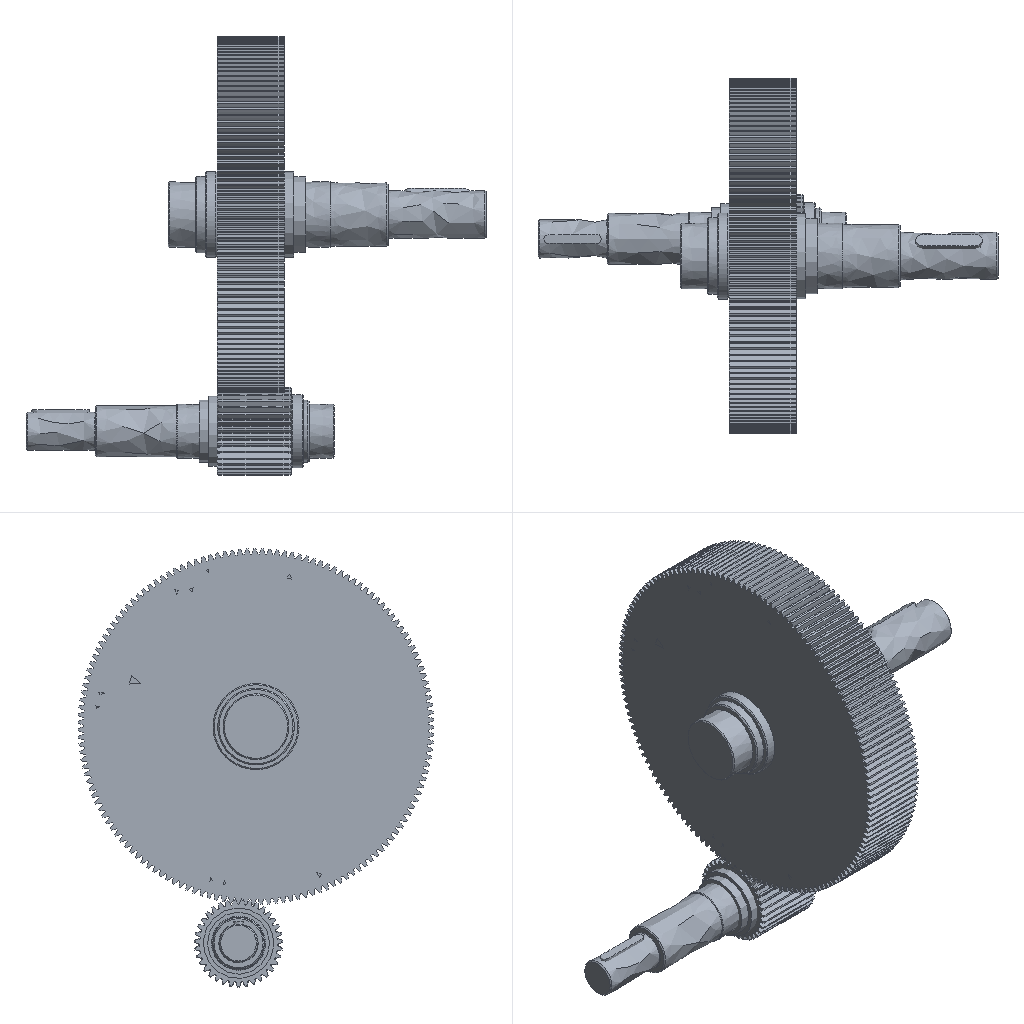Simulation study | ansys workbench
Set-up summary:
category,name,step,type,value,unit,region
solver,ansys_workbench
units,mm-N-s-tonne (MPa),,stated,"/units,MPA"
analysis,LS1,,static
load_step,LS1,LS1,static,nsubst=1; time=1
mesh,nodes,,,107579
mesh,elements,,,52101
element_type,SOLID187,,,31561
element_type,SOLID186,,,8942
element_type,CONTA174,,,5958
element_type,TARGE170,,,5640
material,Structural Steel,,E,200000,tonne s^-2 mm^-1
material,Structural Steel,,nu,0.3
material,Structural Steel,,density,7.85e-09,tonne mm^-3
material,Structural Steel,,conductivity,60.5,tonne mm s^-3 C^-1
material,Structural Steel,,specific_heat,4.34e+08,mm^2 s^-2 C^-1
material,Structural Steel,,cte,1.2e-05,C^-1
material,Structural Steel,,permeability,10000
material,Structural Steel,,resistivity,0.00017,ohm mm
load,,LS1,moment,"500 [dir=(1, 0, 0) n=3]",,all
bc,Fixed Supports,model,fixed,[dofs=ALL],,_FIXEDSU
contact,Contact Region,,bonded (always),element=CONTA174
contact,Contact Region 2,,bonded (always),element=CONTA174
contact,Contact Region 3,,bonded (always),element=CONTA174
contact,Contact Region 4,,bonded (always),element=CONTA174
contact,Contact Region 5,,bonded (always),element=CONTA174
contact,Contact Region 6,,bonded (always),element=CONTA174
contact,Contact Region 7,,bonded (always),element=CONTA174
contact,Contact Region 8,,bonded (always),element=CONTA174
contact,Contact Region 9,,bonded (always),element=CONTA174
contact,Contact Region 10,,bonded (always),element=CONTA174
contact,Contact Region 11,,bonded (always),element=CONTA174
contact,Contact Region 12,,bonded (always),element=CONTA174
contact,Contact Region 13,,bonded (always),element=CONTA174
contact,contact 14,,bonded (always),element=CONTA174
named_set,_FIXEDSU,,node,704
Ansys APDL input file, long lists of numbers shortened:
/batch
/config,noeldb,1     ! force off writing results to database
*get,_wallstrt,active,,time,wall
! ANSYS input file written by Workbench version 2022 R1
! File used for geometry attach:
/title,wbnew--____ (A5)
! ****** Begin Custom Load Command Snippet ******
/COM, ACT Extensions:
/COM,     LSDYNA, 2021.1
/COM,
! ****** End   Custom Load Command Snippet ******
*DIM,_wb_ProjectScratch_dir,string,248
_wb_ProjectScratch_dir(1) = ''
*DIM,_wb_SolverFiles_dir,string,248
_wb_SolverFiles_dir(1) = ''
*DIM,_wb_userfiles_dir,string,248
_wb_userfiles_dir(1) = ''
/com,--- Data in consistent NMM units. See Solving Units in the help system for more information.
/units,MPA
/nopr
/wb,file,start              !  signify a WB generated input file
/prep7
! Turn off shape checking because checks already performed inside WB mesher.
! See help system for more information.
SHPP,OFF,,NOWARN
/nolist
etcon,set             ! allow ANSYS to choose best KEYOP's for 180x elements, resets any applicable keyopt to MAPDL defaults
/com,*********** Nodes for the whole assembly ***********
nblock,3,,118335
(1i9,3e20.9e3)
        1     1.706495079E+02     1.993704432E+00     2.810000000E+01
! (107577 more lines like these left out)
-1
/com,*********** Nodes for all Remote Points ***********
nblock,3
(1i9,3e20.9e3)
   107579     1.897250275E+02    -5.267150244E+00     3.130672649E+01
-1
/wb,elem,start            !  set before creation of elements
/com,*********** Elements for Body 1 "_2___|_ II|__1" ***********
et,1,187
eblock,19,solid,,8572
(19i9)
        1        1        1        1        0        0        0        0       10        0    13585    28511    28512    28794    28787    41030    41045    41038    41036
! (17143 more lines like these left out)
-1
/com,*********** Elements for Body 2 "_2___|GB_T 1096-2003[____ A__ 16_10_46__ 16_10_50|__1" ***********
et,2,186
keyo,2,2,1          ! set full integration on SOLID186
eblock,19,solid,,192
(19i9)
        2        2        2        2        0        0        0        0       20        0      375     1540     1542     1550     1541     1667     1665     1657     1666
! (383 more lines like these left out)
-1
/com,*********** Elements for Body 3 "_2___|__2|__-__1" ***********
et,3,186
keyo,3,2,1          ! set full integration on SOLID186
eblock,19,solid,,8574
(19i9)
        3        3        3        3        0        0        0        0       20        0    22157    41530    44740    44442    42326    48813    47208    47357    48415
! (17147 more lines like these left out)
-1
/com,*********** Elements for Body 4 "_2___|__~_II|__1" ***********
et,4,187
eblock,19,solid,,198
(19i9)
        4        4        4        4        0        0        0        0       10        0      567     2682     2718     2710     2717     3000     3087     2998     2999
! (395 more lines like these left out)
-1
/com,*********** Elements for Body 5 "_2___|GB_T 1096-2003[____ A__ 12_8_70]__ 12_8_70|__1" ***********
et,5,187
eblock,19,solid,,3194
(19i9)
        5        5        5        5        0        0        0        0       10        0      765     3681     3968     4068     4026     7142     8824     7145     7143
! (6387 more lines like these left out)
-1
/com,*********** Elements for Body 6 "_ I|__2" ***********
et,6,187
eblock,19,solid,,7493
(19i9)
        6        6        6        6        0        0        0        0       10        0     6092    14325    15036    15226    15212    21969    26122    21972    21971
! (14985 more lines like these left out)
-1
/com,*********** Elements for Body 7 "___|__-__2" ***********
et,7,187
eblock,19,solid,,9773
(19i9)
        7        7        7        7        0        0        0        0       10        0    30731    90303    90305    92112    91357   100339   100352   100344   100341
! (19545 more lines like these left out)
-1
/com,*********** Elements for Body 8 "GB_T 1096-2003[____ A__ 10_8_50__ 10_8_50|__1" ***********
et,8,187
eblock,19,solid,,2133
(19i9)
        8        8        8        8        0        0        0        0       10        0     3959     9082     9711     9573     9694    10021    12604    10019    10020
! (4265 more lines like these left out)
-1
/com,*********** Elements for Body 9 "GB_T 1096-2003[____ A__ 14_9_56__ 14_9_56|__1" ***********
et,9,186
keyo,9,2,1          ! set full integration on SOLID186
eblock,19,solid,,176
(19i9)
        9        9        9        9        0        0        0        0       20        0        1        1        2        3       12      104      103      102       93
! (351 more lines like these left out)
-1
/com,*********** Elements for Body 10 "__~_I|__1" ***********
et,10,187
eblock,19,solid,,198
(19i9)
       10       10       10       10        0        0        0        0       10        0      177     1062     1082     1081     1071     1246     1324     1245     1243
! (395 more lines like these left out)
-1
/wb,elem,end               !  done creating elements
/com,*********** Send User Defined Coordinate System(s) ***********
csys,0
toffst,273.15,  ! Temperature offset from absolute zero
/com,*********** Set Reference Temperature ***********
tref,22.
/wb,mat,start              !  starting to send materials
/com,*********** Send Materials ***********
Temperature = 'TEMP' ! Temperature
MP,DENS,1,7.85e-09,	! tonne mm^-3
MP,ALPX,1,1.2e-05,	! C^-1
MP,C,1,434000000,	! mm^2 s^-2 C^-1
MP,KXX,1,60.5,	! tonne mm s^-3 C^-1
MP,RSVX,1,0.00017,	! ohm mm
MP,EX,1,200000,	! tonne s^-2 mm^-1
MP,NUXY,1,0.3,
MP,MURX,1,10000,
Temperature = 'TEMP' ! Temperature
MP,DENS,2,7.85e-09,	! tonne mm^-3
MP,ALPX,2,1.2e-05,	! C^-1
MP,C,2,434000000,	! mm^2 s^-2 C^-1
MP,KXX,2,60.5,	! tonne mm s^-3 C^-1
MP,RSVX,2,0.00017,	! ohm mm
MP,EX,2,200000,	! tonne s^-2 mm^-1
MP,NUXY,2,0.3,
MP,MURX,2,10000,
Temperature = 'TEMP' ! Temperature
MP,DENS,3,7.85e-09,	! tonne mm^-3
MP,ALPX,3,1.2e-05,	! C^-1
MP,C,3,434000000,	! mm^2 s^-2 C^-1
MP,KXX,3,60.5,	! tonne mm s^-3 C^-1
MP,RSVX,3,0.00017,	! ohm mm
MP,EX,3,200000,	! tonne s^-2 mm^-1
MP,NUXY,3,0.3,
MP,MURX,3,10000,
Temperature = 'TEMP' ! Temperature
MP,DENS,4,7.85e-09,	! tonne mm^-3
MP,ALPX,4,1.2e-05,	! C^-1
MP,C,4,434000000,	! mm^2 s^-2 C^-1
MP,KXX,4,60.5,	! tonne mm s^-3 C^-1
MP,RSVX,4,0.00017,	! ohm mm
MP,EX,4,200000,	! tonne s^-2 mm^-1
MP,NUXY,4,0.3,
MP,MURX,4,10000,
Temperature = 'TEMP' ! Temperature
MP,DENS,5,7.85e-09,	! tonne mm^-3
MP,ALPX,5,1.2e-05,	! C^-1
MP,C,5,434000000,	! mm^2 s^-2 C^-1
MP,KXX,5,60.5,	! tonne mm s^-3 C^-1
MP,RSVX,5,0.00017,	! ohm mm
MP,EX,5,200000,	! tonne s^-2 mm^-1
MP,NUXY,5,0.3,
MP,MURX,5,10000,
Temperature = 'TEMP' ! Temperature
MP,DENS,6,7.85e-09,	! tonne mm^-3
MP,ALPX,6,1.2e-05,	! C^-1
MP,C,6,434000000,	! mm^2 s^-2 C^-1
MP,KXX,6,60.5,	! tonne mm s^-3 C^-1
MP,RSVX,6,0.00017,	! ohm mm
MP,EX,6,200000,	! tonne s^-2 mm^-1
MP,NUXY,6,0.3,
MP,MURX,6,10000,
Temperature = 'TEMP' ! Temperature
MP,DENS,7,7.85e-09,	! tonne mm^-3
MP,ALPX,7,1.2e-05,	! C^-1
MP,C,7,434000000,	! mm^2 s^-2 C^-1
MP,KXX,7,60.5,	! tonne mm s^-3 C^-1
MP,RSVX,7,0.00017,	! ohm mm
MP,EX,7,200000,	! tonne s^-2 mm^-1
MP,NUXY,7,0.3,
MP,MURX,7,10000,
Temperature = 'TEMP' ! Temperature
MP,DENS,8,7.85e-09,	! tonne mm^-3
MP,ALPX,8,1.2e-05,	! C^-1
MP,C,8,434000000,	! mm^2 s^-2 C^-1
MP,KXX,8,60.5,	! tonne mm s^-3 C^-1
MP,RSVX,8,0.00017,	! ohm mm
MP,EX,8,200000,	! tonne s^-2 mm^-1
MP,NUXY,8,0.3,
MP,MURX,8,10000,
Temperature = 'TEMP' ! Temperature
MP,DENS,9,7.85e-09,	! tonne mm^-3
MP,ALPX,9,1.2e-05,	! C^-1
MP,C,9,434000000,	! mm^2 s^-2 C^-1
MP,KXX,9,60.5,	! tonne mm s^-3 C^-1
MP,RSVX,9,0.00017,	! ohm mm
MP,EX,9,200000,	! tonne s^-2 mm^-1
MP,NUXY,9,0.3,
MP,MURX,9,10000,
Temperature = 'TEMP' ! Temperature
MP,DENS,10,7.85e-09,	! tonne mm^-3
MP,ALPX,10,1.2e-05,	! C^-1
MP,C,10,434000000,	! mm^2 s^-2 C^-1
MP,KXX,10,60.5,	! tonne mm s^-3 C^-1
MP,RSVX,10,0.00017,	! ohm mm
MP,EX,10,200000,	! tonne s^-2 mm^-1
MP,NUXY,10,0.3,
MP,MURX,10,10000,
/wb,mat,end                !  done sending materials
!************************* Model Summary ********************
!_2___|_ II|__1,	结构钢,	matid,	1
!_2___|GB_T 1096-2003[____ A__ 16_10_46__ 16_10_50|__1,	结构钢,	matid,	2
!_2___|__2|__-__1,	结构钢,	matid,	3
!_2___|__~_II|__1,	结构钢,	matid,	4
!_2___|GB_T 1096-2003[____ A__ 12_8_70]__ 12_8_70|__1,	结构钢,	matid,	5
!_ I|__2,	结构钢,	matid,	6
!___|__-__2,	结构钢,	matid,	7
!GB_T 1096-2003[____ A__ 10_8_50__ 10_8_50|__1,	结构钢,	matid,	8
!GB_T 1096-2003[____ A__ 14_9_56__ 14_9_56|__1,	结构钢,	matid,	9
!__~_I|__1,	结构钢,	matid,	10
!************************* End Model Summary ********************
! get the diagonal of the bounding box. Needed later for other things
*get,_xmin,node,,mnloc,x
*get,_ymin,node,,mnloc,y
*get,_zmin,node,,mnloc,z
*get,_xmax,node,,mxloc,x
*get,_ymax,node,,mxloc,y
*get,_zmax,node,,mxloc,z
_ASMDIAG=(_xmax-_xmin)*(_xmax-_xmin)+(_ymax-_ymin)*(_ymax-_ymin)+(_zmax-_zmin)*(_zmax-_zmin)
_ASMDIAG=SQRT(_ASMDIAG)
/wb,contact,start          !  starting to send contact
/com,*********** Create Contact "接触区域" ***********
/com,            Real Constant Set For Above Contact Is 12 & 11
*set,tid,12
*set,cid,11
r,tid
r,cid
et,tid,170
et,cid,174
eblock,10,,,46
(15i9)
    63849       12       12       12        0    26772    26768    26773    26773    31125    31126    26773    31154
! (45 more lines like these left out)
-1
eblock,10,,,46
(15i9)
    63895       11       11       11        0    26772    26768    26773    26773    31125    31126    26773    31154
! (45 more lines like these left out)
-1
eblock,10,,,150
(15i9)
    63941       11       12       11        0     1727     1711     1720     1719     2385     2383     2407     2408
! (149 more lines like these left out)
-1
eblock,10,,,150
(15i9)
    64091       12       11       12        0     1727     1711     1720     1719     2385     2383     2407     2408
! (149 more lines like these left out)
-1
keyo,cid,8,2               ! auto create asymmetric contact (from Program Controlled setting)
keyo,cid,10,0              ! adjust contact stiffness each NR iteration (from Program Controlled setting)
keyo,cid,12,5              ! bonded always
keyo,cid,18,1              ! small sliding turned on by application
keyo,cid,2,0               ! augmented Lagrange (from Program Controlled setting)
keyo,cid,4,0               ! on Gauss point (from Program Controlled setting)
keyo,cid,9,1               ! ignore initial gaps/penetration
keyo,cid,7,0               ! No Prediction
rmod,tid,3,10.      ! FKN
rmod,tid,5,0.       ! ICONT
rmod,tid,6,0.       ! PINB
rmod,tid,10,0.      ! CNOF
rmod,tid,12,0.      ! FKT
rmod,tid,36,53      ! WB DSID
rmod,cid,3,10.      ! FKN
rmod,cid,5,0.       ! ICONT
rmod,cid,6,0.       ! PINB
rmod,cid,10,0.      ! CNOF
rmod,cid,12,0.      ! FKT
rmod,cid,36,53      ! WB DSID
/com,*********** Create Contact "接触区域 2" ***********
/com,            Real Constant Set For Above Contact Is 14 & 13
*set,tid,14
*set,cid,13
r,tid
r,cid
et,tid,170
et,cid,174
eblock,10,,,557
(15i9)
    64241       14       14       14        0    26368    26375    27732    27732    28892    28986    27732    28899
! (556 more lines like these left out)
-1
eblock,10,,,557
(15i9)
    64798       13       13       13        0    26368    26375    27732    27732    28892    28986    27732    28899
! (556 more lines like these left out)
-1
eblock,10,,,56
(15i9)
    65355       13       14       13        0    52103    52092    52098    52099    84320    84319    84331    84333
! (55 more lines like these left out)
-1
eblock,10,,,56
(15i9)
    65411       14       13       14        0    52103    52092    52098    52099    84320    84319    84331    84333
! (55 more lines like these left out)
-1
keyo,cid,8,2               ! auto create asymmetric contact (from Program Controlled setting)
keyo,cid,10,0              ! adjust contact stiffness each NR iteration (from Program Controlled setting)
keyo,cid,12,5              ! bonded always
keyo,cid,18,1              ! small sliding turned on by application
keyo,cid,2,0               ! augmented Lagrange (from Program Controlled setting)
keyo,cid,4,0               ! on Gauss point (from Program Controlled setting)
keyo,cid,9,1               ! ignore initial gaps/penetration
keyo,cid,7,0               ! No Prediction
rmod,tid,3,10.      ! FKN
rmod,tid,5,0.       ! ICONT
rmod,tid,6,0.       ! PINB
rmod,tid,10,0.      ! CNOF
rmod,tid,12,0.      ! FKT
rmod,tid,36,56      ! WB DSID
rmod,cid,3,10.      ! FKN
rmod,cid,5,0.       ! ICONT
rmod,cid,6,0.       ! PINB
rmod,cid,10,0.      ! CNOF
rmod,cid,12,0.      ! FKT
rmod,cid,36,56      ! WB DSID
/com,*********** Create Contact "接触区域 3" ***********
/com,            Real Constant Set For Above Contact Is 16 & 15
*set,tid,16
*set,cid,15
r,tid
r,cid
et,tid,170
et,cid,174
eblock,10,,,144
(15i9)
    65467       16       16       16        0    27296    27687    28003    28003    34416    36123    28003    34417
! (143 more lines like these left out)
-1
eblock,10,,,144
(15i9)
    65611       15       15       15        0    27296    27687    28003    28003    34416    36123    28003    34417
! (143 more lines like these left out)
-1
eblock,10,,,32
(15i9)
    65755       15       16       15        0     2669     2678     2671     2671     2921     2929     2671     2920
! (31 more lines like these left out)
-1
eblock,10,,,32
(15i9)
    65787       16       15       16        0     2669     2678     2671     2671     2921     2929     2671     2920
! (31 more lines like these left out)
-1
keyo,cid,8,2               ! auto create asymmetric contact (from Program Controlled setting)
keyo,cid,10,0              ! adjust contact stiffness each NR iteration (from Program Controlled setting)
keyo,cid,12,5              ! bonded always
keyo,cid,18,1              ! small sliding turned on by application
keyo,cid,2,0               ! augmented Lagrange (from Program Controlled setting)
keyo,cid,4,0               ! on Gauss point (from Program Controlled setting)
keyo,cid,9,1               ! ignore initial gaps/penetration
keyo,cid,7,0               ! No Prediction
rmod,tid,3,10.      ! FKN
rmod,tid,5,0.       ! ICONT
rmod,tid,6,0.       ! PINB
rmod,tid,10,0.      ! CNOF
rmod,tid,12,0.      ! FKT
rmod,tid,36,59      ! WB DSID
rmod,cid,3,10.      ! FKN
rmod,cid,5,0.       ! ICONT
rmod,cid,6,0.       ! PINB
rmod,cid,10,0.      ! CNOF
rmod,cid,12,0.      ! FKT
rmod,cid,36,59      ! WB DSID
/com,*********** Create Contact "接触区域 4" ***********
/com,            Real Constant Set For Above Contact Is 18 & 17
*set,tid,18
*set,cid,17
r,tid
r,cid
et,tid,170
et,cid,174
eblock,10,,,44
(15i9)
    65819       18       18       18        0    26778    26774    26779    26779    31174    31175    26779    31195
! (43 more lines like these left out)
-1
eblock,10,,,44
(15i9)
    65863       17       17       17        0    26778    26774    26779    26779    31174    31175    26779    31195
! (43 more lines like these left out)
-1
eblock,10,,,954
(15i9)
    65907       17       18       17        0     3139     3374     3382     3382     4208     5781     3382     4209
! (953 more lines like these left out)
-1
eblock,10,,,954
(15i9)
    66861       18       17       18        0     3139     3374     3382     3382     4208     5781     3382     4209
! (953 more lines like these left out)
-1
keyo,cid,8,2               ! auto create asymmetric contact (from Program Controlled setting)
keyo,cid,10,0              ! adjust contact stiffness each NR iteration (from Program Controlled setting)
keyo,cid,12,5              ! bonded always
keyo,cid,18,1              ! small sliding turned on by application
keyo,cid,2,0               ! augmented Lagrange (from Program Controlled setting)
keyo,cid,4,0               ! on Gauss point (from Program Controlled setting)
keyo,cid,9,1               ! ignore initial gaps/penetration
keyo,cid,7,0               ! No Prediction
rmod,tid,3,10.      ! FKN
rmod,tid,5,0.       ! ICONT
rmod,tid,6,0.       ! PINB
rmod,tid,10,0.      ! CNOF
rmod,tid,12,0.      ! FKT
rmod,tid,36,62      ! WB DSID
rmod,cid,3,10.      ! FKN
rmod,cid,5,0.       ! ICONT
rmod,cid,6,0.       ! PINB
rmod,cid,10,0.      ! CNOF
rmod,cid,12,0.      ! FKT
rmod,cid,36,62      ! WB DSID
/com,*********** Create Contact "接触区域 5" ***********
/com,            Real Constant Set For Above Contact Is 20 & 19
*set,tid,20
*set,cid,19
r,tid
r,cid
et,tid,170
et,cid,174
eblock,10,,,150
(15i9)
    67815       20       20       20        0     1699     1700     1709     1710     2356     2359     2378     2357
! (149 more lines like these left out)
-1
eblock,10,,,150
(15i9)
    67965       19       19       19        0     1699     1700     1709     1710     2356     2359     2378     2357
! (149 more lines like these left out)
-1
eblock,10,,,12
(15i9)
    68115       19       20       19        0    54641    54640    54638    54635    89019    89017    89013    89014
! (11 more lines like these left out)
-1
eblock,10,,,12
(15i9)
    68127       20       19       20        0    54641    54640    54638    54635    89019    89017    89013    89014
! (11 more lines like these left out)
-1
keyo,cid,8,2               ! auto create asymmetric contact (from Program Controlled setting)
keyo,cid,10,0              ! adjust contact stiffness each NR iteration (from Program Controlled setting)
keyo,cid,12,5              ! bonded always
keyo,cid,18,1              ! small sliding turned on by application
keyo,cid,2,0               ! augmented Lagrange (from Program Controlled setting)
keyo,cid,4,0               ! on Gauss point (from Program Controlled setting)
keyo,cid,9,1               ! ignore initial gaps/penetration
keyo,cid,7,0               ! No Prediction
rmod,tid,3,10.      ! FKN
rmod,tid,5,0.       ! ICONT
rmod,tid,6,0.       ! PINB
rmod,tid,10,0.      ! CNOF
rmod,tid,12,0.      ! FKT
rmod,tid,36,65      ! WB DSID
rmod,cid,3,10.      ! FKN
rmod,cid,5,0.       ! ICONT
rmod,cid,6,0.       ! PINB
rmod,cid,10,0.      ! CNOF
rmod,cid,12,0.      ! FKT
rmod,cid,36,65      ! WB DSID
/com,*********** Create Contact "接触区域 6" ***********
/com,            Real Constant Set For Above Contact Is 22 & 21
*set,tid,22
*set,cid,21
r,tid
r,cid
et,tid,170
et,cid,174
eblock,10,,,27
(15i9)
    68139       22       22       22        0    48243    48759    48254    48789    76861    76882    76883    76862
! (26 more lines like these left out)
-1
eblock,10,,,27
(15i9)
    68166       21       21       21        0    48243    48759    48254    48789    76861    76882    76883    76862
! (26 more lines like these left out)
-1
eblock,10,,,32
(15i9)
    68193       21       22       21        0     2682     2701     2702     2702     2996     3052     2702     2997
! (31 more lines like these left out)
-1
eblock,10,,,32
(15i9)
    68225       22       21       22        0     2682     2701     2702     2702     2996     3052     2702     2997
! (31 more lines like these left out)
-1
keyo,cid,8,2               ! auto create asymmetric contact (from Program Controlled setting)
keyo,cid,10,0              ! adjust contact stiffness each NR iteration (from Program Controlled setting)
keyo,cid,12,5              ! bonded always
keyo,cid,18,1              ! small sliding turned on by application
keyo,cid,2,0               ! augmented Lagrange (from Program Controlled setting)
keyo,cid,4,0               ! on Gauss point (from Program Controlled setting)
keyo,cid,9,1               ! ignore initial gaps/penetration
keyo,cid,7,0               ! No Prediction
rmod,tid,3,10.      ! FKN
rmod,tid,5,0.       ! ICONT
rmod,tid,6,0.       ! PINB
rmod,tid,10,0.      ! CNOF
rmod,tid,12,0.      ! FKT
rmod,tid,36,68      ! WB DSID
rmod,cid,3,10.      ! FKN
rmod,cid,5,0.       ! ICONT
rmod,cid,6,0.       ! PINB
rmod,cid,10,0.      ! CNOF
rmod,cid,12,0.      ! FKT
rmod,cid,36,68      ! WB DSID
/com,*********** Create Contact "接触区域 7" ***********
/com,            Real Constant Set For Above Contact Is 24 & 23
*set,tid,24
*set,cid,23
r,tid
r,cid
et,tid,170
et,cid,174
eblock,10,,,51
(15i9)
    68257       24       24       24        0    52658    52661    52657    52656    85632    85629    85626    85627
! (50 more lines like these left out)
-1
eblock,10,,,51
(15i9)
    68308       23       23       23        0    52658    52661    52657    52656    85632    85629    85626    85627
! (50 more lines like these left out)
-1
eblock,10,,,300
(15i9)
    68359       23       24       23        0    89360    90371    90359    90359    94249   100564    90359    94248
! (299 more lines like these left out)
-1
eblock,10,,,300
(15i9)
    68659       24       23       24        0    89360    90371    90359    90359    94249   100564    90359    94248
! (299 more lines like these left out)
-1
keyo,cid,8,2               ! auto create asymmetric contact (from Program Controlled setting)
keyo,cid,10,0              ! adjust contact stiffness each NR iteration (from Program Controlled setting)
keyo,cid,12,5              ! bonded always
keyo,cid,18,1              ! small sliding turned on by application
keyo,cid,2,0               ! augmented Lagrange (from Program Controlled setting)
keyo,cid,4,0               ! on Gauss point (from Program Controlled setting)
keyo,cid,9,1               ! ignore initial gaps/penetration
keyo,cid,7,0               ! No Prediction
rmod,tid,3,10.      ! FKN
rmod,tid,5,0.       ! ICONT
rmod,tid,6,0.       ! PINB
rmod,tid,10,0.      ! CNOF
rmod,tid,12,0.      ! FKT
rmod,tid,36,71      ! WB DSID
rmod,cid,3,10.      ! FKN
rmod,cid,5,0.       ! ICONT
rmod,cid,6,0.       ! PINB
rmod,cid,10,0.      ! CNOF
rmod,cid,12,0.      ! FKT
rmod,cid,36,71      ! WB DSID
/com,*********** Create Contact "接触区域 8" ***********
/com,            Real Constant Set For Above Contact Is 26 & 25
*set,tid,26
*set,cid,25
r,tid
r,cid
et,tid,170
et,cid,174
eblock,10,,,572
(15i9)
    68959       26       26       26        0    14300    14296    14016    14016    21826    20532    14016    20533
! (571 more lines like these left out)
-1
eblock,10,,,572
(15i9)
    69531       25       25       25        0    14300    14296    14016    14016    21826    20532    14016    20533
! (571 more lines like these left out)
-1
eblock,10,,,617
(15i9)
    70103       25       26       25        0    89327    89328    90325    90325    94035    94043    90325    94039
! (616 more lines like these left out)
-1
eblock,10,,,617
(15i9)
    70720       26       25       26        0    89327    89328    90325    90325    94035    94043    90325    94039
! (616 more lines like these left out)
-1
keyo,cid,8,2               ! auto create asymmetric contact (from Program Controlled setting)
keyo,cid,10,0              ! adjust contact stiffness each NR iteration (from Program Controlled setting)
keyo,cid,12,5              ! bonded always
keyo,cid,18,1              ! small sliding turned on by application
keyo,cid,2,0               ! augmented Lagrange (from Program Controlled setting)
keyo,cid,4,0               ! on Gauss point (from Program Controlled setting)
keyo,cid,9,1               ! ignore initial gaps/penetration
keyo,cid,7,0               ! No Prediction
rmod,tid,3,10.      ! FKN
rmod,tid,5,0.       ! ICONT
rmod,tid,6,0.       ! PINB
rmod,tid,10,0.      ! CNOF
rmod,tid,12,0.      ! FKT
rmod,tid,36,74      ! WB DSID
rmod,cid,3,10.      ! FKN
rmod,cid,5,0.       ! ICONT
rmod,cid,6,0.       ! PINB
rmod,cid,10,0.      ! CNOF
rmod,cid,12,0.      ! FKT
rmod,cid,36,74      ! WB DSID
/com,*********** Create Contact "接触区域 9" ***********
/com,            Real Constant Set For Above Contact Is 28 & 27
*set,tid,28
*set,cid,27
r,tid
r,cid
et,tid,170
et,cid,174
eblock,10,,,44
(15i9)
    71337       28       28       28        0    13453    13452    13448    13448    17227    17203    13448    17204
! (43 more lines like these left out)
-1
eblock,10,,,44
(15i9)
    71381       27       27       27        0    13453    13452    13448    13448    17227    17203    13448    17204
! (43 more lines like these left out)
-1
eblock,10,,,690
(15i9)
    71425       27       28       27        0     9275     9063     9167     9167     9888     9887     9167    10549
! (689 more lines like these left out)
-1
eblock,10,,,690
(15i9)
    72115       28       27       28        0     9275     9063     9167     9167     9888     9887     9167    10549
! (689 more lines like these left out)
-1
keyo,cid,8,2               ! auto create asymmetric contact (from Program Controlled setting)
keyo,cid,10,0              ! adjust contact stiffness each NR iteration (from Program Controlled setting)
keyo,cid,12,5              ! bonded always
keyo,cid,18,1              ! small sliding turned on by application
keyo,cid,2,0               ! augmented Lagrange (from Program Controlled setting)
keyo,cid,4,0               ! on Gauss point (from Program Controlled setting)
keyo,cid,9,1               ! ignore initial gaps/penetration
keyo,cid,7,0               ! No Prediction
rmod,tid,3,10.      ! FKN
rmod,tid,5,0.       ! ICONT
rmod,tid,6,0.       ! PINB
rmod,tid,10,0.      ! CNOF
rmod,tid,12,0.      ! FKT
rmod,tid,36,77      ! WB DSID
rmod,cid,3,10.      ! FKN
rmod,cid,5,0.       ! ICONT
rmod,cid,6,0.       ! PINB
rmod,cid,10,0.      ! CNOF
rmod,cid,12,0.      ! FKT
rmod,cid,36,77      ! WB DSID
/com,*********** Create Contact "接触区域 10" ***********
/com,            Real Constant Set For Above Contact Is 30 & 29
*set,tid,30
*set,cid,29
r,tid
r,cid
et,tid,170
et,cid,174
eblock,10,,,44
(15i9)
    72805       30       30       30        0    13216    13212    13217    13217    15999    16000    13217    16033
! (43 more lines like these left out)
-1
eblock,10,,,44
(15i9)
    72849       29       29       29        0    13216    13212    13217    13217    15999    16000    13217    16033
! (43 more lines like these left out)
-1
eblock,10,,,154
(15i9)
    72893       29       30       29        0      181      168      176      175      820      819      832      833
! (153 more lines like these left out)
-1
eblock,10,,,154
(15i9)
    73047       30       29       30        0      181      168      176      175      820      819      832      833
! (153 more lines like these left out)
-1
keyo,cid,8,2               ! auto create asymmetric contact (from Program Controlled setting)
keyo,cid,10,0              ! adjust contact stiffness each NR iteration (from Program Controlled setting)
keyo,cid,12,5              ! bonded always
keyo,cid,18,1              ! small sliding turned on by application
keyo,cid,2,0               ! augmented Lagrange (from Program Controlled setting)
keyo,cid,4,0               ! on Gauss point (from Program Controlled setting)
keyo,cid,9,1               ! ignore initial gaps/penetration
keyo,cid,7,0               ! No Prediction
rmod,tid,3,10.      ! FKN
rmod,tid,5,0.       ! ICONT
rmod,tid,6,0.       ! PINB
rmod,tid,10,0.      ! CNOF
rmod,tid,12,0.      ! FKT
rmod,tid,36,80      ! WB DSID
rmod,cid,3,10.      ! FKN
rmod,cid,5,0.       ! ICONT
rmod,cid,6,0.       ! PINB
rmod,cid,10,0.      ! CNOF
rmod,cid,12,0.      ! FKT
rmod,cid,36,80      ! WB DSID
/com,*********** Create Contact "接触区域 11" ***********
/com,            Real Constant Set For Above Contact Is 32 & 31
*set,tid,32
*set,cid,31
r,tid
r,cid
et,tid,170
et,cid,174
eblock,10,,,138
(15i9)
    73201       32       32       32        0    13469    14223    14547    14547    17390    21466    14547    17391
! (137 more lines like these left out)
-1
eblock,10,,,138
(15i9)
    73339       31       31       31        0    13469    14223    14547    14547    17390    21466    14547    17391
! (137 more lines like these left out)
-1
eblock,10,,,32
(15i9)
    73477       31       32       31        0     1086     1095     1088     1088     1338     1346     1088     1337
! (31 more lines like these left out)
-1
eblock,10,,,32
(15i9)
    73509       32       31       32        0     1086     1095     1088     1088     1338     1346     1088     1337
! (31 more lines like these left out)
-1
keyo,cid,8,2               ! auto create asymmetric contact (from Program Controlled setting)
keyo,cid,10,0              ! adjust contact stiffness each NR iteration (from Program Controlled setting)
keyo,cid,12,5              ! bonded always
keyo,cid,18,1              ! small sliding turned on by application
keyo,cid,2,0               ! augmented Lagrange (from Program Controlled setting)
keyo,cid,4,0               ! on Gauss point (from Program Controlled setting)
keyo,cid,9,1               ! ignore initial gaps/penetration
keyo,cid,7,0               ! No Prediction
rmod,tid,3,10.      ! FKN
rmod,tid,5,0.       ! ICONT
rmod,tid,6,0.       ! PINB
rmod,tid,10,0.      ! CNOF
rmod,tid,12,0.      ! FKT
rmod,tid,36,83      ! WB DSID
rmod,cid,3,10.      ! FKN
rmod,cid,5,0.       ! ICONT
rmod,cid,6,0.       ! PINB
rmod,cid,10,0.      ! CNOF
rmod,cid,12,0.      ! FKT
rmod,cid,36,83      ! WB DSID
/com,*********** Create Contact "接触区域 12" ***********
/com,            Real Constant Set For Above Contact Is 34 & 33
*set,tid,34
*set,cid,33
r,tid
r,cid
et,tid,170
et,cid,174
eblock,10,,,52
(15i9)
    73541       34       34       34        0    89044    91311    90036    90036    92413    99210    90036    92411
! (51 more lines like these left out)
-1
eblock,10,,,52
(15i9)
    73593       33       33       33        0    89044    91311    90036    90036    92413    99210    90036    92411
! (51 more lines like these left out)
-1
eblock,10,,,162
(15i9)
    73645       33       34       33        0      181      168      176      175      820      819      832      833
! (161 more lines like these left out)
-1
eblock,10,,,162
(15i9)
    73807       34       33       34        0      181      168      176      175      820      819      832      833
! (161 more lines like these left out)
-1
keyo,cid,8,2               ! auto create asymmetric contact (from Program Controlled setting)
keyo,cid,10,0              ! adjust contact stiffness each NR iteration (from Program Controlled setting)
keyo,cid,12,5              ! bonded always
keyo,cid,18,1              ! small sliding turned on by application
keyo,cid,2,0               ! augmented Lagrange (from Program Controlled setting)
keyo,cid,4,0               ! on Gauss point (from Program Controlled setting)
keyo,cid,9,1               ! ignore initial gaps/penetration
keyo,cid,7,0               ! No Prediction
rmod,tid,3,10.      ! FKN
rmod,tid,5,0.       ! ICONT
rmod,tid,6,0.       ! PINB
rmod,tid,10,0.      ! CNOF
rmod,tid,12,0.      ! FKT
rmod,tid,36,86      ! WB DSID
rmod,cid,3,10.      ! FKN
rmod,cid,5,0.       ! ICONT
rmod,cid,6,0.       ! PINB
rmod,cid,10,0.      ! CNOF
rmod,cid,12,0.      ! FKT
rmod,cid,36,86      ! WB DSID
/com,*********** Create Contact "接触区域 13" ***********
/com,            Real Constant Set For Above Contact Is 36 & 35
*set,tid,36
*set,cid,35
r,tid
r,cid
et,tid,170
et,cid,174
eblock,10,,,548
(15i9)
    73969       36       36       36        0    91443    91512    91501    91501   105521   105757    91501   105519
! (547 more lines like these left out)
-1
eblock,10,,,548
(15i9)
    74517       35       35       35        0    91443    91512    91501    91501   105521   105757    91501   105519
! (547 more lines like these left out)
-1
eblock,10,,,32
(15i9)
    75065       35       36       35        0     1100     1120     1121     1121     1422     1477     1121     1423
! (31 more lines like these left out)
-1
eblock,10,,,32
(15i9)
    75097       36       35       36        0     1100     1120     1121     1121     1422     1477     1121     1423
! (31 more lines like these left out)
-1
keyo,cid,8,2               ! auto create asymmetric contact (from Program Controlled setting)
keyo,cid,10,0              ! adjust contact stiffness each NR iteration (from Program Controlled setting)
keyo,cid,12,5              ! bonded always
keyo,cid,18,1              ! small sliding turned on by application
keyo,cid,2,0               ! augmented Lagrange (from Program Controlled setting)
keyo,cid,4,0               ! on Gauss point (from Program Controlled setting)
keyo,cid,9,1               ! ignore initial gaps/penetration
keyo,cid,7,0               ! No Prediction
rmod,tid,3,10.      ! FKN
rmod,tid,5,0.       ! ICONT
rmod,tid,6,0.       ! PINB
rmod,tid,10,0.      ! CNOF
rmod,tid,12,0.      ! FKT
rmod,tid,36,89      ! WB DSID
rmod,cid,3,10.      ! FKN
rmod,cid,5,0.       ! ICONT
rmod,cid,6,0.       ! PINB
rmod,cid,10,0.      ! CNOF
rmod,cid,12,0.      ! FKT
rmod,cid,36,89      ! WB DSID
nsel,all
esel,all
/wb,contact,end            !  done creating contacts
/golist
/wb,load,start             !  starting to send loads
/com,*********** Fixed Supports ***********
CMBLOCK,_FIXEDSU,NODE,      704
(8i10)
     13194     13196     13197     13198     13231     13232     13233     13234
! (87 more lines like these left out)
cmsel,s,_FIXEDSU
d,all,all
nsel,all
/com,*********** Create Remote Point "内部远程点" ***********
! -------- Remote Point Used by "力矩" --------
*set,tid,38
*set,cid,37
et,cid,174
et,tid,170
keyo,tid,2,1               ! Don't fix the pilot node
keyo,tid,4,111111
keyo,cid,12,5              ! Bonded Contact
keyo,cid,4,1               ! Deformable RBE3 style load
keyo,cid,2,2               ! MPC style contact
eblock,10,,,318
(15i9)
    75129       37       37       37        0    53632    53628    53630    53631    87437    87436    87441    87443
! (317 more lines like these left out)
-1
*set,_npilot,107579
_npilot100=_npilot
type,tid
mat ,cid
real,cid
tshape,pilo
en,75447,_npilot
tshape
/com,*********** Construct Moment Using Remote Attachment ***********
/gst,on,on
fini
*get,_numnode,node,0,count
*get,_numelem,elem,0,count
*get, _MAXELEMNUM, elem, 0, NUM, MAX
*get, _MAXNODENUM, node, 0, NUM, MAX
*get, _MAXELEMTYPE, etyp, 0, NUM, MAX
*get, _MAXREALCONST, real, 0, NUM, MAX
/go
/wb,load,end               !  done creating loads
/com,--- Number of total nodes = %_numnode%
/com,--- Number of contact elements = 11598
/com,--- Number of spring elements = 0
/com,--- Number of bearing elements = 0
/com,--- Number of solid elements = 40503
/com,--- Number of condensed parts = 0
/com,--- Number of total elements = %_numelem%
*get,_wallbsol,active,,time,wall
/com,****************************************************************************
/com,*************************    SOLUTION       ********************************
/com,****************************************************************************
/solu
antype,0                   ! static analysis
_thickRatio=0.8     ! Ratio of thick parts in the model
eqsl,pcg,1e-8,,,,,,1
cntr,print,1               ! print out contact info and also make no initial contact an error
dmpoption,emat,no             ! Don't combine emat file for DANSYS
dmpoption,esav,no             ! Don't combine esav file for DANSYS
nldiag,cont,iter           ! print out contact info each equilibrium iteration
rescontrol,,none                 ! Do not keep any restart files
/com,****************************************************
/com,******************* SOLVE FOR LS 1 OF 1 ****************
nsel,s,node,,107579
f,all,mx,500.
f,all,my,0.
f,all,mz,0.
nsel,all
/nopr
/gopr
nsub,1,1,1
time,1.
outres,erase
outres,all,none
outres,nsol,all,
outres,rsol,all
outres,eangl,all
outres,etmp,all
outres,veng,all
outres,strs,all,
outres,epel,all,
outres,eppl,all,
outres,cont,all,
! *********** WB SOLVE COMMAND ***********
! check interactive state
*get,ANSINTER_,active,,int
*if,ANSINTER_,ne,0,then
/eof
*endif
solve
/com *************** Write FE CONNECTORS *********
CEWRITE,file,ce,,INTE
/com,****************************************************
/com,*************** FINISHED SOLVE FOR LS 1 *************
*get,_wallasol,active,,time,wall
/nopr
*get,_numnode,node,0,count
*get,_numelem,elem,0,count
*get, _MAXELEMNUM, elem, 0, NUM, MAX
*get, _MAXNODENUM, node, 0, NUM, MAX,,,INTERNAL
*get, _MAXELEMTYPE, etyp, 0, NUM, MAX
*get, _MAXREALCONST, real, 0, NUM, MAX
/gopr
*get,_PCGITER,active,,solu,cgiter
/post1
xmlo,ENCODING,ISO-8859-1
xmlo,parm
/xml,parm,xml
fini
/gopr
*get,_walldone,active,,time,wall
_preptime=(_wallbsol-_wallstrt)*3600
_solvtime=(_wallasol-_wallbsol)*3600
_posttime=(_walldone-_wallasol)*3600
_totaltim=(_walldone-_wallstrt)*3600
*get,_dlbratio,active,0,solu,dlbr
*get,_combtime,active,0,solu,comb
*get,_ssmode,active,0,solu,ssmm
*get,_ndofs,active,0,solu,ndof
*get,_sol_end_time,active,0,set,time
*if,_sol_end_time,eq,1.,then
/fclean				!clean distributed files
*endif
/com,--- Total number of nodes = %_numnode%
/com,--- Total number of elements = %_numelem%
/com,--- Element load balance ratio = %_dlbratio%
/com,--- Time to combine distributed files = %_combtime%
/com,--- Sparse memory mode = %_ssmode%
/com,--- Number of DOF = %_ndofs%
/wb,file,end               ! done with WB generated input
Results summary:
result,analyses[0].index,,,1
result,analyses[0].system,,,SYS
result,analyses[0].deck,,,deck.dat
result,analyses[0].solve_status,,,completed
result,analyses[0].analysis_type,,,static
result,analyses[0].physics,,,mechanical
result,analyses[0].unit_system,,,"NMM: mm, ton, N, s, mV, mA, degC"
result,analyses[0].n_sets,,,1
result,analyses[0].load_steps[0].set,set=1,,1
result,analyses[0].load_steps[0].time_or_freq,set=1,,1
result,analyses[0].load_steps[0].max_displacement_magnitude,set=1,,5.69838e-05
result,analyses[0].load_steps[0].max_von_mises_nodal,set=1,,0.2024
result,analyses[0].load_steps[0].reaction_force_sum_xyz[1],set=1,,-2.78241e-06
result,analyses[0].load_steps[0].reaction_force_sum_xyz[2],set=1,,6.34373e-08
result,analyses[0].load_steps[0].reaction_force_sum_xyz[3],set=1,,-4.55316e-07